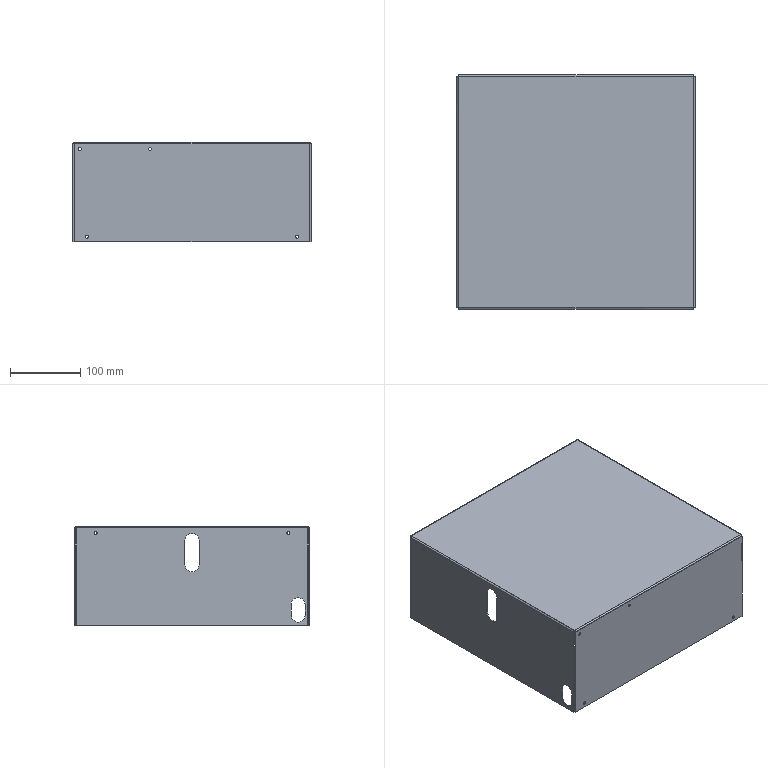Part | NX | features BREP 1 | 1 solid | 66 faces | box 340 x 335 x 142 mm | volume 445198 mm3 | plane 30 | cylinder 28 | spline 8 | commonest cylinder face diameters 4.2 x8 20 x8 1.473 x4 4.3 x4 4.473 x4